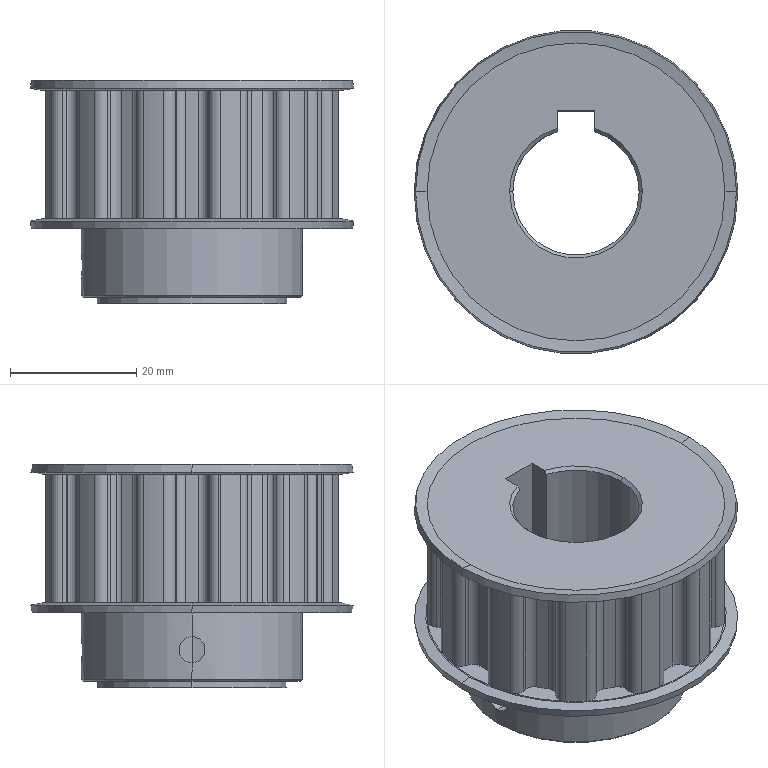Part | STEP file | Timing pulley 1_3 | 1 solid | 172 faces | box 51.203 x 51.203 x 35.319 mm | volume 36393 mm3 | cylinder 81 | plane 67 | cone 20 | spline 4 | commonest cylinder face diameters 3.2 x58 47.139 x12 4.134 x4 20 x3 30 x2 35 x2